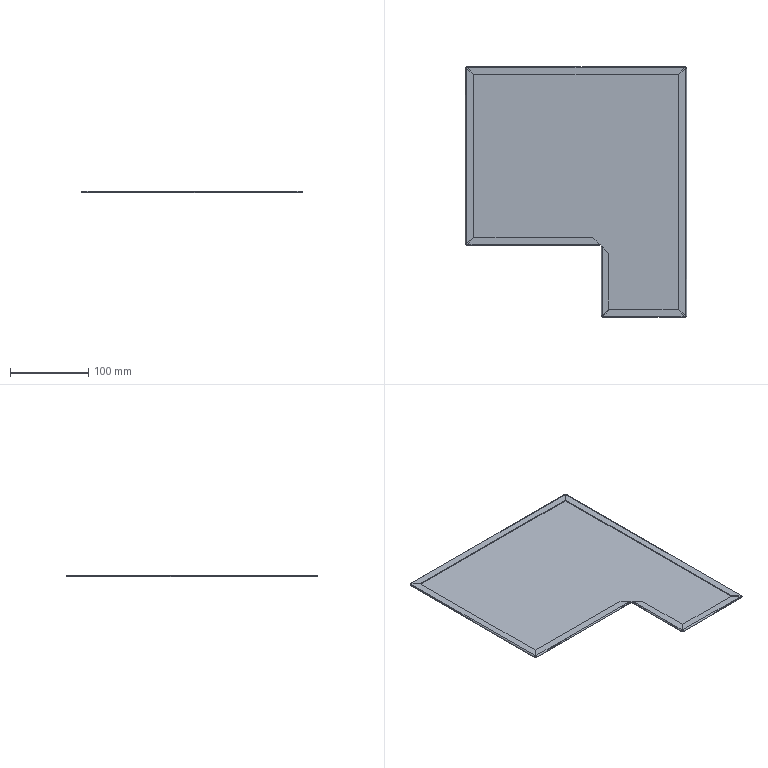Part | STEP file | Guide wheel mechanism revised.sldasm-Part-333 | 1 solid | 57 faces | box 282 x 320 x 2.5 mm | volume 102141 mm3 | plane 33 | spline 12 | cylinder 12 | commonest cylinder face diameters 0.1 x6 2.5 x6